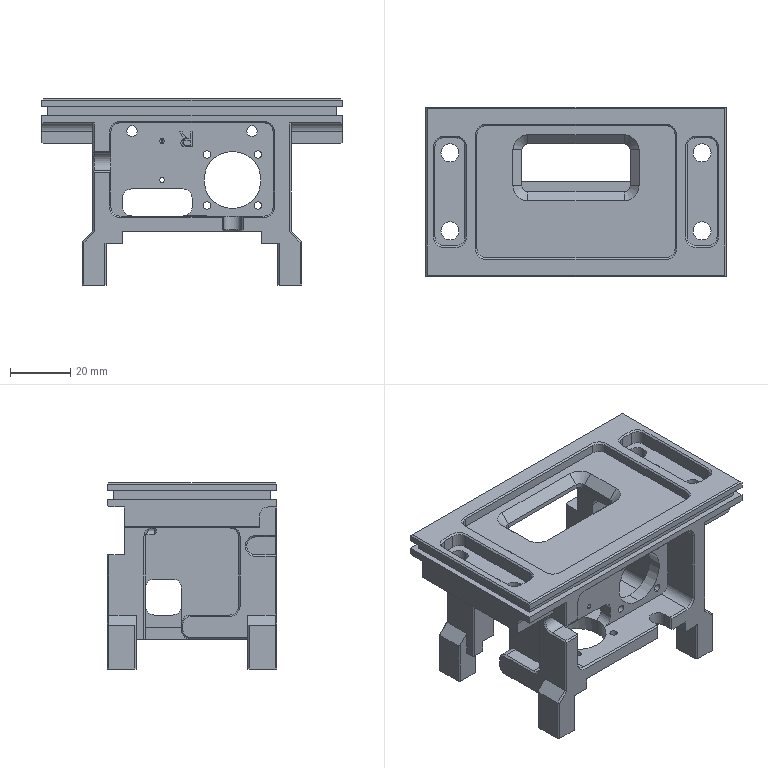NC program | Mastercam | posted with a generic post | part box 100 x 56.5 x 62 mm
Lines 34 to 1353 of 45570:
N260 T13 M6
N270 G0 G90 G17 G54 X-61.557 Y-50.411 A0. S5500 M3
N280 G43 H13 Z20. M8
N290 Z1.
N300 G1 Z-28.25 F600.
N310 X-62.09 Y-49.087 Z-28.374 F3000.
N320 G3 X-62.884 Y-47.884 Z-28.5 I-3.34 J-1.343
N330 G1 X-63.092 Y-47.603
N340 X-63.557 Y-46.951
N350 X-63.842 Y-46.52
N360 X-64.135 Y-46.037
N370 X-64.424 Y-45.51
N380 X-64.698 Y-44.943
N390 X-64.951 Y-44.341
N400 X-65.173 Y-43.718
N410 X-65.349 Y-43.127
N420 X-65.486 Y-42.577
N430 X-65.592 Y-42.064
N440 X-65.674 Y-41.586
N450 X-65.738 Y-41.138
N460 X-65.826 Y-40.34
N470 X-65.882 Y-39.609
N480 X-65.918 Y-38.931
N490 X-65.941 Y-38.291
N500 X-65.956 Y-37.678
N510 X-65.965 Y-37.084
N520 X-65.971 Y-36.505
N530 X-65.974 Y-35.935
N540 X-65.975 Y-35.371
N550 X-65.976 Y-34.813
N560 X-65.975 Y-34.258
N570 X-65.974 Y-33.705
N580 X-65.973 Y-33.153
N590 X-65.972 Y-32.603
N600 X-65.971 Y-32.052
N610 X-65.969 Y-31.502
N620 X-65.967 Y-30.953
N630 X-65.966 Y-30.403
N640 X-65.964 Y-29.853
N650 X-65.963 Y-29.304
N660 X-65.961 Y-28.754
N670 X-65.959 Y-28.205
N680 X-65.958 Y-27.655
N690 X-65.956 Y-27.105
N700 X-65.955 Y-26.556
N710 X-65.953 Y-26.006
N720 X-65.951 Y-25.456
N730 X-65.95 Y-24.906
N740 X-65.948 Y-24.357
N750 X-65.946 Y-23.807
N760 X-65.945 Y-23.257
N770 X-65.943 Y-22.707
N780 X-65.942 Y-22.157
N790 X-65.94 Y-21.607
N800 X-65.938 Y-21.057
N810 X-65.937 Y-20.507
N820 X-65.935 Y-19.957
N830 X-65.933 Y-19.407
N840 X-65.932 Y-18.857
N850 X-65.93 Y-18.307
N860 X-65.929 Y-17.757
N870 X-65.927 Y-17.207
N880 X-65.925 Y-16.656
N890 X-65.924 Y-16.106
N900 X-65.922 Y-15.556
N910 X-65.92 Y-15.006
N920 X-65.919 Y-14.456
N930 X-65.917 Y-13.905
N940 X-65.916 Y-13.355
N950 X-65.914 Y-12.805
N960 X-65.912 Y-12.254
N970 X-65.911 Y-11.704
N980 X-65.909 Y-11.153
N990 X-65.907 Y-10.603
N1000 X-65.906 Y-10.052
N1010 X-65.904 Y-9.502
N1020 X-65.903 Y-8.951
N1030 X-65.901 Y-8.401
N1040 X-65.899 Y-7.85
N1050 X-65.898 Y-7.3
N1060 X-65.896 Y-6.749
N1070 X-65.894 Y-6.199
N1080 X-65.893 Y-5.648
N1090 X-65.891 Y-5.097
N1100 X-65.89 Y-4.547
N1110 X-65.888 Y-3.996
N1120 X-65.886 Y-3.445
N1130 X-65.885 Y-2.895
N1140 X-65.883 Y-2.344
N1150 X-65.881 Y-1.793
N1160 X-65.88 Y-1.242
N1170 X-65.878 Y-.691
N1180 X-65.877 Y-.141
N1190 X-65.875 Y.41
N1200 X-65.873 Y.961
N1210 X-65.872 Y1.512
N1220 X-65.87 Y2.063
N1230 X-65.868 Y2.614
N1240 X-65.867 Y3.165
N1250 X-65.865 Y3.716
N1260 X-65.863 Y4.267
N1270 X-65.862 Y4.818
N1280 X-65.86 Y5.369
N1290 X-65.859 Y5.92
N1300 X-65.857 Y6.471
N1310 X-65.855 Y7.022
N1320 X-65.854 Y7.573
N1330 X-65.852 Y8.124
N1340 X-65.85 Y8.675
N1350 X-65.849 Y9.226
N1360 X-65.847 Y9.778
N1370 X-65.846 Y10.329
N1380 X-65.844 Y10.88
N1390 X-65.842 Y11.431
N1400 X-65.841 Y11.982
N1410 X-65.839 Y12.534
N1420 X-65.837 Y13.085
N1430 X-65.836 Y13.636
N1440 X-65.834 Y14.187
N1450 X-65.833 Y14.739
N1460 X-65.831 Y15.29
N1470 X-65.829 Y15.841
N1480 X-65.828 Y16.393
N1490 X-65.826 Y16.944
N1500 X-65.824 Y17.495
N1510 X-65.823 Y18.047
N1520 X-65.821 Y18.598
N1530 X-65.819 Y19.149
N1540 X-65.818 Y19.701
N1550 X-65.816 Y20.252
N1560 X-65.815 Y20.804
N1570 X-65.813 Y21.355
N1580 X-65.811 Y21.907
N1590 X-65.81 Y22.458
N1600 X-65.808 Y23.01
N1610 X-65.806 Y23.561
N1620 X-65.805 Y24.113
N1630 X-65.803 Y24.664
N1640 X-65.802 Y25.216
N1650 X-65.8 Y25.767
N1660 X-65.798 Y26.319
N1670 X-65.797 Y26.871
N1680 X-65.795 Y27.422
N1690 X-65.793 Y27.974
N1700 X-65.792 Y28.525
N1710 X-65.79 Y29.077
N1720 X-65.788 Y29.629
N1730 X-65.787 Y30.18
N1740 X-65.785 Y30.732
N1750 X-65.784 Y31.284
N1760 X-65.782 Y31.836
N1770 X-65.78 Y32.387
N1780 X-65.779 Y32.939
N1790 X-65.777 Y33.491
N1800 X-65.775 Y34.043
N1810 X-65.774 Y34.594
N1820 X-65.772 Y35.146
N1830 X-65.771 Y35.698
N1840 X-65.769 Y36.25
N1850 X-65.767 Y36.802
N1860 X-65.766 Y37.353
N1870 X-65.763 Y37.956
N1880 X-65.741 Y38.755
N1890 X-65.712 Y39.225
N1900 X-65.664 Y39.727
N1910 X-65.595 Y40.255
N1920 X-65.501 Y40.803
N1930 X-65.378 Y41.367
N1940 X-65.225 Y41.941
N1950 X-65.038 Y42.521
N1960 X-64.816 Y43.103
N1970 X-64.558 Y43.682
N1980 X-64.263 Y44.254
N1990 X-63.93 Y44.815
N2000 X-63.561 Y45.361
N2010 X-63.155 Y45.888
N2020 X-62.713 Y46.394
N2030 X-62.236 Y46.873
N2040 X-61.727 Y47.322
N2050 X-61.206 Y47.726
N2060 X-60.682 Y48.086
N2070 X-60.159 Y48.403
N2080 X-59.642 Y48.683
N2090 X-59.134 Y48.928
N2100 X-58.637 Y49.142
N2110 X-58.152 Y49.33
N2120 X-57.68 Y49.493
N2130 X-57.221 Y49.635
N2140 X-56.775 Y49.759
N2150 X-56.343 Y49.867
N2160 X-55.531 Y50.041
N2170 X-54.76 Y50.176
N2180 X-54.023 Y50.28
N2190 X-53.317 Y50.361
N2200 X-52.638 Y50.424
N2210 X-51.981 Y50.473
N2220 X-51.343 Y50.511
N2230 X-50.721 Y50.542
N2240 X-50.111 Y50.565
N2250 X-49.512 Y50.584
N2260 X-48.922 Y50.598
N2270 X-48.338 Y50.609
N2280 X-47.761 Y50.618
N2290 X-47.189 Y50.624
N2300 X-46.62 Y50.629
N2310 X-46.054 Y50.633
N2320 X-45.49 Y50.636
N2330 X-44.927 Y50.639
N2340 X-44.365 Y50.641
N2350 X-43.804 Y50.642
N2360 X-43.243 Y50.644
N2370 X-42.684 Y50.645
N2380 X-42.124 Y50.646
N2390 X-41.566 Y50.647
N2400 X-41.007
N2410 X-40.449 Y50.648
N2420 X-39.891
N2430 X-39.333
N2440 X-38.776 Y50.649
N2450 X-38.218
N2460 X-37.661
N2470 X-37.104
N2480 X-36.546
N2490 X-35.989 Y50.65
N2500 X-35.432
N2510 X-34.875
N2520 X-34.318
N2530 X-33.761
N2540 X-33.204
N2550 X-32.647
N2560 X-32.09
N2570 X-31.533
N2580 X-30.976
N2590 X-30.419
N2600 X-29.862
N2610 X-29.305
N2620 X-28.748
N2630 X-28.191
N2640 X-27.634
N2650 X-27.077
N2660 X-26.521
N2670 X-25.964
N2680 X-25.407
N2690 X-24.85
N2700 X-24.293
N2710 X-23.736
N2720 X-23.179
N2730 X-22.622
N2740 X-22.065
N2750 X-21.508
N2760 X-20.951
N2770 X-20.394
N2780 X-19.838
N2790 X-19.281
N2800 X-18.724
N2810 X-18.167
N2820 X-17.61
N2830 X-17.053
N2840 X-16.496
N2850 X-15.939
N2860 X-15.382
N2870 X-14.825
N2880 X-14.268
N2890 X-13.712
N2900 X-13.155
N2910 X-12.598
N2920 X-12.041
N2930 X-11.484
N2940 X-10.927
N2950 X-10.37
N2960 X-9.813
N2970 X-9.256
N2980 X-8.699
N2990 X-8.142
N3000 X-7.586
N3010 X-7.029
N3020 X-6.472
N3030 X-5.915
N3040 X-5.358
N3050 X-4.801
N3060 X-4.244
N3070 X-3.687
N3080 X-3.13
N3090 X-2.573
N3100 X-2.016
N3110 X-1.46
N3120 X-.903
N3130 X-.346
N3140 X.211
N3150 X.768
N3160 X1.325
N3170 X1.882
N3180 X2.439
N3190 X2.996
N3200 X3.553
N3210 X4.11
N3220 X4.667
N3230 X5.223
N3240 X5.78
N3250 X6.337
N3260 X6.894
N3270 X7.451
N3280 X8.008
N3290 X8.565
N3300 X9.122
N3310 X9.679
N3320 X10.236
N3330 X10.793
N3340 X11.349
N3350 X11.906
N3360 X12.463
N3370 X13.02
N3380 X13.577
N3390 X14.134
N3400 X14.691
N3410 X15.248
N3420 X15.805
N3430 X16.362
N3440 X16.919
N3450 X17.475
N3460 X18.032
N3470 X18.589
N3480 X19.146
N3490 X19.703
N3500 X20.26
N3510 X20.817
N3520 X21.374
N3530 X21.931
N3540 X22.488
N3550 X23.045
N3560 X23.601
N3570 X24.158
N3580 X24.715
N3590 X25.272
N3600 X25.829
N3610 X26.386
N3620 X26.943
N3630 X27.5
N3640 X28.057
N3650 X28.614
N3660 X29.171
N3670 X29.727
N3680 X30.284
N3690 X30.841
N3700 X31.398
N3710 X31.955
N3720 X32.512
N3730 X33.069
N3740 X33.626
N3750 X34.183
N3760 X34.74
N3770 X35.297
N3780 X35.853
N3790 X36.41
N3800 X36.967
N3810 X37.524
N3820 X38.081
N3830 X38.638
N3840 X39.195
N3850 X39.752
N3860 X40.309
N3870 X40.866
N3880 X41.423
N3890 X41.979
N3900 X42.536
N3910 X43.093
N3920 X43.65
N3930 X44.207
N3940 X44.764
N3950 X45.321
N3960 X45.878
N3970 X46.435
N3980 X46.992
N3990 X47.549
N4000 X48.106
N4010 X48.662
N4020 X49.219
N4030 X49.776
N4040 X50.333
N4050 X50.89
N4060 X51.447
N4070 X52.004
N4080 X52.602 Y50.649
N4090 X53.378 Y50.633
N4100 X53.831 Y50.61
N4110 X54.315 Y50.571
N4120 X54.825 Y50.513
N4130 X55.356 Y50.432
N4140 X55.903 Y50.326
N4150 X56.462 Y50.192
N4160 X57.028 Y50.026
N4170 X57.599 Y49.829
N4180 X58.169 Y49.597
N4190 X58.735 Y49.331
N4200 X59.292 Y49.028
N4210 X59.838 Y48.69
N4220 X60.369 Y48.315
N4230 X60.881 Y47.905
N4240 X61.37 Y47.46
N4250 X61.832 Y46.983
N4260 X62.253 Y46.49
N4270 X62.634 Y45.988
N4280 X62.975 Y45.483
N4290 X63.28 Y44.978
N4300 X63.552 Y44.478
N4310 X63.793 Y43.983
N4320 X64.006 Y43.498
N4330 X64.194 Y43.021
N4340 X64.36 Y42.556
N4350 X64.507 Y42.102
N4360 X64.636 Y41.659
N4370 X64.75 Y41.227
N4380 X64.936 Y40.413
N4390 X65.081 Y39.635
N4400 X65.196 Y38.891
N4410 X65.286 Y38.176
N4420 X65.358 Y37.487
N4430 X65.415 Y36.82
N4440 X65.46 Y36.172
N4450 X65.496 Y35.539
N4460 X65.526 Y34.92
N4470 X65.549 Y34.311
N4480 X65.568 Y33.712
N4490 X65.583 Y33.12
N4500 X65.596 Y32.534
N4510 X65.606 Y31.954
N4520 X65.614 Y31.378
N4530 X65.621 Y30.805
N4540 X65.626 Y30.235
N4550 X65.63 Y29.668
N4560 X65.634 Y29.102
N4570 X65.637 Y28.538
N4580 X65.639 Y27.975
N4590 X65.641 Y27.413
N4600 X65.643 Y26.853
N4610 X65.644 Y26.292
N4620 X65.645 Y25.733
N4630 X65.646 Y25.174
N4640 X65.647 Y24.615
N4650 Y24.057
N4660 X65.648 Y23.499
N4670 Y22.941
N4680 X65.649 Y22.383
N4690 Y21.826
N4700 Y21.268
N4710 Y20.711
N4720 Y20.154
N4730 Y19.596
N4740 X65.65 Y19.039
N4750 Y18.482
N4760 Y17.925
N4770 Y17.368
N4780 Y16.811
N4790 Y16.254
N4800 Y15.697
N4810 Y15.14
N4820 Y14.583
N4830 Y14.026
N4840 Y13.469
N4850 Y12.912
N4860 Y12.355
N4870 Y11.798
N4880 Y11.241
N4890 Y10.684
N4900 Y10.128
N4910 Y9.571
N4920 Y9.014
N4930 Y8.457
N4940 Y7.9
N4950 Y7.343
N4960 Y6.786
N4970 Y6.229
N4980 Y5.672
N4990 Y5.115
N5000 Y4.558
N5010 Y4.001
N5020 Y3.445
N5030 Y2.888
N5040 Y2.331
N5050 Y1.774
N5060 Y1.217
N5070 Y.66
N5080 Y.103
N5090 Y-.454
N5100 Y-1.011
N5110 Y-1.568
N5120 Y-2.125
N5130 Y-2.681
N5140 Y-3.238
N5150 Y-3.795
N5160 Y-4.352
N5170 Y-4.909
N5180 Y-5.466
N5190 Y-6.023
N5200 Y-6.58
N5210 Y-7.137
N5220 Y-7.694
N5230 Y-8.251
N5240 Y-8.807
N5250 Y-9.364
N5260 Y-9.921
N5270 Y-10.478
N5280 Y-11.035
N5290 Y-11.592
N5300 Y-12.149
N5310 Y-12.706
N5320 Y-13.263
N5330 Y-13.82
N5340 Y-14.377
N5350 Y-14.933
N5360 Y-15.49
N5370 Y-16.047
N5380 Y-16.604
N5390 Y-17.161
N5400 Y-17.718
N5410 Y-18.275
N5420 Y-18.832
N5430 Y-19.389
N5440 Y-19.946
N5450 Y-20.503
N5460 Y-21.06
N5470 Y-21.616
N5480 Y-22.173
N5490 Y-22.73
N5500 Y-23.287
N5510 Y-23.844
N5520 Y-24.401
N5530 Y-24.958
N5540 Y-25.515
N5550 Y-26.072
N5560 Y-26.629
N5570 Y-27.186
N5580 Y-27.742
N5590 Y-28.299
N5600 Y-28.856
N5610 Y-29.413
N5620 Y-29.97
N5630 Y-30.527
N5640 Y-31.084
N5650 Y-31.641
N5660 Y-32.198
N5670 Y-32.755
N5680 Y-33.312
N5690 Y-33.868
N5700 Y-34.425
N5710 Y-34.982
N5720 Y-35.539
N5730 Y-36.096
N5740 Y-36.653
N5750 Y-37.21
N5760 X65.646 Y-37.871
N5770 X65.618 Y-38.703
N5780 X65.583 Y-39.179
N5790 X65.531 Y-39.682
N5800 X65.457 Y-40.207
N5810 X65.358 Y-40.75
N5820 X65.232 Y-41.306
N5830 X65.075 Y-41.871
N5840 X64.887 Y-42.441
N5850 X64.665 Y-43.011
N5860 X64.408 Y-43.579
N5870 X64.116 Y-44.139
N5880 X63.787 Y-44.689
N5890 X63.422 Y-45.224
N5900 X63.022 Y-45.741
N5910 X62.587 Y-46.237
N5920 X62.117 Y-46.708
N5930 X61.628 Y-47.141
N5940 X61.128 Y-47.533
N5950 X60.623 Y-47.885
N5960 X60.118 Y-48.199
N5970 X59.616 Y-48.48
N5980 X59.119 Y-48.729
N5990 X58.631 Y-48.95
N6000 X58.152 Y-49.145
N6010 X57.684 Y-49.317
N6020 X57.226 Y-49.468
N6030 X56.78 Y-49.602
N6040 X56.345 Y-49.72
N6050 X55.921 Y-49.824
N6060 X55.121 Y-49.994
N6070 X54.356 Y-50.127
N6080 X53.624 Y-50.232
N6090 X52.919 Y-50.315
N6100 X52.238 Y-50.381
N6110 X51.578 Y-50.433
N6120 X50.936 Y-50.475
N6130 X50.309 Y-50.508
N6140 X49.693 Y-50.535
N6150 X49.089 Y-50.556
N6160 X48.492 Y-50.574
N6170 X47.903 Y-50.588
N6180 X47.319 Y-50.6
N6190 X46.74 Y-50.609
N6200 X46.165 Y-50.616
N6210 X45.594 Y-50.623
N6220 X45.025 Y-50.628
N6230 X44.458 Y-50.632
N6240 X43.893 Y-50.635
N6250 X43.329 Y-50.638
N6260 X42.767 Y-50.64
N6270 X42.206 Y-50.642
N6280 X41.645 Y-50.643
N6290 X41.085 Y-50.645
N6300 X40.526 Y-50.646
N6310 X39.967
N6320 X39.409 Y-50.647
N6330 X38.85 Y-50.648
N6340 X38.292
N6350 X37.735
N6360 X37.177 Y-50.649
N6370 X36.619
N6380 X36.062
N6390 X35.505
N6400 X34.947
N6410 X34.39
N6420 X33.833 Y-50.65
N6430 X33.276
N6440 X32.719
N6450 X32.162
N6460 X31.605
N6470 X31.048
N6480 X30.491
N6490 X29.934
N6500 X29.377
N6510 X28.82
N6520 X28.263
N6530 X27.706
N6540 X27.149
N6550 X26.592
N6560 X26.035
N6570 X25.478
N6580 X24.921
N6590 X24.364
N6600 X23.808
N6610 X23.251
N6620 X22.694
N6630 X22.137
N6640 X21.58
N6650 X21.023
N6660 X20.466
N6670 X19.909
N6680 X19.352
N6690 X18.795
N6700 X18.238
N6710 X17.682
N6720 X17.125
N6730 X16.568
N6740 X16.011
N6750 X15.454
N6760 X14.897
N6770 X14.34
N6780 X13.783
N6790 X13.226
N6800 X12.669
N6810 X12.112
N6820 X11.555
N6830 X10.999
N6840 X10.442
N6850 X9.885
N6860 X9.328
N6870 X8.771
N6880 X8.214
N6890 X7.657
N6900 X7.1
N6910 X6.543
N6920 X5.986
N6930 X5.429
N6940 X4.873
N6950 X4.316
N6960 X3.759
N6970 X3.202
N6980 X2.645
N6990 X2.088
N7000 X1.531
N7010 X.974
N7020 X.417
N7030 X-.14
N7040 X-.697
N7050 X-1.253
N7060 X-1.81
N7070 X-2.367
N7080 X-2.924
N7090 X-3.481
N7100 X-4.038
N7110 X-4.595
N7120 X-5.152
N7130 X-5.709
N7140 X-6.266
N7150 X-6.823
N7160 X-7.379
N7170 X-7.936
N7180 X-8.493
N7190 X-9.05
N7200 X-9.607
N7210 X-10.164
N7220 X-10.721
N7230 X-11.278
N7240 X-11.835
N7250 X-12.392
N7260 X-12.949
N7270 X-13.505
N7280 X-14.062
N7290 X-14.619
N7300 X-15.176
N7310 X-15.733
N7320 X-16.29
N7330 X-16.847
N7340 X-17.404
N7350 X-17.961
N7360 X-18.518
N7370 X-19.075
N7380 X-19.631
N7390 X-20.188
N7400 X-20.745
N7410 X-21.302
N7420 X-21.859
N7430 X-22.416
N7440 X-22.973
N7450 X-23.53
N7460 X-24.087
N7470 X-24.644
N7480 X-25.201
N7490 X-25.758
N7500 X-26.314
N7510 X-26.871
N7520 X-27.428
N7530 X-27.985
N7540 X-28.542
N7550 X-29.099
N7560 X-29.656
N7570 X-30.213
N7580 X-30.77
N7590 X-31.327
N7600 X-31.884
N7610 X-32.44
N7620 X-32.997
N7630 X-33.554
N7640 X-34.111
N7650 X-34.668
N7660 X-35.225
N7670 X-35.782
N7680 X-36.339
N7690 X-36.896
N7700 X-37.453
N7710 X-38.01
N7720 X-38.566
N7730 X-39.123
N7740 X-39.68
N7750 X-40.237
N7760 X-40.794
N7770 X-41.351
N7780 X-41.908
N7790 X-42.465
N7800 X-43.022
N7810 X-43.579
N7820 X-44.136
N7830 X-44.692
N7840 X-45.249
N7850 X-45.806
N7860 X-46.363
N7870 X-46.92
N7880 X-47.477
N7890 X-48.034
N7900 X-48.591
N7910 X-49.148
N7920 X-49.705
N7930 X-50.262
N7940 X-50.818
N7950 X-51.375
N7960 X-51.932
N7970 X-52.515
N7980 X-53.27 Y-50.637
N7990 X-53.714 Y-50.617
N8000 X-54.191 Y-50.582
N8010 X-54.695 Y-50.529
N8020 X-55.221 Y-50.455
N8030 X-55.809 Y-50.345
N8040 X-56.451 Y-50.186
N8050 X-57.077 Y-49.989
N8060 X-57.687 Y-49.755
N8070 X-58.281 Y-49.484
N8080 X-58.857 Y-49.178
N8090 X-59.414 Y-48.837
N8100 X-59.948 Y-48.462
N8110 X-60.455 Y-48.059
N8120 X-60.931 Y-47.632
N8130 X-61.376 Y-47.184
N8140 X-61.787 Y-46.722
N8150 X-62.164 Y-46.251
N8160 X-62.509 Y-45.771
N8170 X-62.823 Y-45.289
N8180 X-63.108 Y-44.805
N8190 X-63.364 Y-44.323
N8200 X-63.595 Y-43.845
N8210 X-63.801 Y-43.374
N8220 X-63.986 Y-42.909
N8230 X-64.15 Y-42.452
N8240 X-64.297 Y-42.005
N8250 X-64.427 Y-41.566
N8260 X-64.543 Y-41.137
N8270 X-64.733 Y-40.325
N8280 X-64.884 Y-39.546
N8290 X-65.003 Y-38.798
N8300 X-65.098 Y-38.078
N8310 X-65.172 Y-37.383
N8320 X-65.231 Y-36.711
N8330 X-65.278 Y-36.057
N8340 X-65.315 Y-35.42
N8350 X-65.345 Y-34.796
N8360 X-65.368 Y-34.184
N8370 X-65.387 Y-33.582
N8380 X-65.402 Y-32.988
N8390 X-65.413 Y-32.4
N8400 X-65.422 Y-31.818
N8410 X-65.43 Y-31.24
N8420 X-65.435 Y-30.666
N8430 X-65.439 Y-30.095
N8440 X-65.442 Y-29.527
N8450 X-65.444 Y-28.961
N8460 X-65.446 Y-28.396
N8470 X-65.447 Y-27.833
N8480 Y-27.271
N8490 Y-26.71
N8500 Y-26.149
N8510 Y-25.589
N8520 X-65.446 Y-25.03
N8530 X-65.445 Y-24.471
N8540 X-65.444 Y-23.913
N8550 X-65.443 Y-23.355
N8560 X-65.442 Y-22.797
N8570 X-65.44 Y-22.239
N8580 X-65.439 Y-21.682
N8590 X-65.438 Y-21.124
N8600 X-65.436 Y-20.567
N8610 X-65.435 Y-20.009
N8620 X-65.433 Y-19.452
N8630 X-65.431 Y-18.895
N8640 X-65.43 Y-18.338
N8650 X-65.428 Y-17.781
N8660 X-65.427 Y-17.224
N8670 X-65.425 Y-16.667
N8680 X-65.424 Y-16.11
N8690 X-65.422 Y-15.553
N8700 X-65.42 Y-14.996
N8710 X-65.419 Y-14.439
N8720 X-65.417 Y-13.882
N8730 X-65.415 Y-13.325
N8740 X-65.414 Y-12.768
N8750 X-65.412 Y-12.211
N8760 X-65.41 Y-11.654
N8770 X-65.409 Y-11.097
N8780 X-65.407 Y-10.54
N8790 X-65.406 Y-9.983
N8800 X-65.404 Y-9.426
N8810 X-65.402 Y-8.869
N8820 X-65.401 Y-8.312
N8830 X-65.399 Y-7.756
N8840 X-65.397 Y-7.199
N8850 X-65.396 Y-6.642
N8860 X-65.394 Y-6.085
N8870 X-65.392 Y-5.528
N8880 X-65.391 Y-4.971
N8890 X-65.389 Y-4.414
N8900 X-65.387 Y-3.857
N8910 X-65.386 Y-3.3
N8920 X-65.384 Y-2.743
N8930 X-65.383 Y-2.186
N8940 X-65.381 Y-1.63
N8950 X-65.379 Y-1.073
N8960 X-65.378 Y-.516
N8970 X-65.376 Y.041
N8980 X-65.374 Y.598
N8990 X-65.373 Y1.155
N9000 X-65.371 Y1.712
N9010 X-65.369 Y2.269
N9020 X-65.368 Y2.826
N9030 X-65.366 Y3.383
N9040 X-65.364 Y3.94
N9050 X-65.363 Y4.496
N9060 X-65.361 Y5.053
N9070 X-65.359 Y5.61
N9080 X-65.358 Y6.167
N9090 X-65.356 Y6.724
N9100 X-65.355 Y7.281
N9110 X-65.353 Y7.838
N9120 X-65.351 Y8.395
N9130 X-65.35 Y8.952
N9140 X-65.348 Y9.509
N9150 X-65.346 Y10.066
N9160 X-65.345 Y10.622
N9170 X-65.343 Y11.179
N9180 X-65.341 Y11.736
N9190 X-65.34 Y12.293
N9200 X-65.338 Y12.85
N9210 X-65.336 Y13.407
N9220 X-65.335 Y13.964
N9230 X-65.333 Y14.521
N9240 X-65.331 Y15.078
N9250 X-65.33 Y15.635
N9260 X-65.328 Y16.192
N9270 X-65.327 Y16.748
N9280 X-65.325 Y17.305
N9290 X-65.323 Y17.862
N9300 X-65.322 Y18.419
N9310 X-65.32 Y18.976
N9320 X-65.318 Y19.533
N9330 X-65.317 Y20.09
N9340 X-65.315 Y20.647
N9350 X-65.313 Y21.204
N9360 X-65.312 Y21.761
N9370 X-65.31 Y22.318
N9380 X-65.308 Y22.874
N9390 X-65.307 Y23.431
N9400 X-65.305 Y23.988
N9410 X-65.304 Y24.545
N9420 X-65.302 Y25.102
N9430 X-65.3 Y25.659
N9440 X-65.299 Y26.216
N9450 X-65.297 Y26.773
N9460 X-65.295 Y27.33
N9470 X-65.294 Y27.887
N9480 X-65.292 Y28.443
N9490 X-65.29 Y29.
N9500 X-65.289 Y29.557
N9510 X-65.287 Y30.114
N9520 X-65.285 Y30.671
N9530 X-65.284 Y31.228
N9540 X-65.282 Y31.785
N9550 X-65.28 Y32.342
N9560 X-65.279 Y32.899
N9570 X-65.277 Y33.456
N9580 X-65.276 Y34.013
N9590 X-65.274 Y34.57
N9600 X-65.272 Y35.132
N9610 X-65.269 Y35.722
N9620 X-65.259 Y36.383
N9630 X-65.231 Y37.133
N9640 X-65.204 Y37.555
N9650 X-65.165 Y38.001
N9660 X-65.111 Y38.477
N9670 X-65.038 Y38.977
N9680 X-64.941 Y39.503
N9690 X-64.817 Y40.047
N9700 X-64.661 Y40.613
N9710 X-64.472 Y41.188
N9720 X-64.247 Y41.765
N9730 X-63.989 Y42.333
N9740 X-63.699 Y42.888
N9750 X-63.379 Y43.425
N9760 X-63.032 Y43.94
N9770 X-62.662 Y44.431
N9780 X-62.271 Y44.896
N9790 X-61.862 Y45.334
N9800 X-61.435 Y45.748
N9810 X-61.003 Y46.129
N9820 X-60.558 Y46.486
N9830 X-60.112 Y46.813
N9840 X-59.658 Y47.118
N9850 X-59.206 Y47.396
N9860 X-58.75 Y47.653
N9870 X-58.3 Y47.886
N9880 X-57.85 Y48.1
N9890 X-57.407 Y48.294
N9900 X-56.966 Y48.471
N9910 X-56.534 Y48.631
N9920 X-56.106 Y48.777
N9930 X-55.687 Y48.908
N9940 X-54.883 Y49.131
N9950 X-54.105 Y49.315
N9960 X-53.35 Y49.465
N9970 X-52.619 Y49.588
N9980 X-51.91 Y49.689
N9990 X-51.221 Y49.772
N100 X-50.55 Y49.839
N110 X-49.895 Y49.895
N120 X-49.255 Y49.94
N130 X-48.627 Y49.977
N140 X-48.011 Y50.007
N150 X-47.404 Y50.032
N160 X-46.805 Y50.052
N170 X-46.213 Y50.069
N180 X-45.627 Y50.083
N190 X-45.045 Y50.095
N200 X-44.468 Y50.104
N210 X-43.894 Y50.112
N220 X-43.323 Y50.118
N230 X-42.754 Y50.124
N240 X-42.187 Y50.128
N250 X-41.622 Y50.132
N260 X-41.058 Y50.135
N270 X-40.495 Y50.138
N280 X-39.933 Y50.14
N290 X-39.373 Y50.142
N300 X-38.812 Y50.143
N310 X-38.253 Y50.144
N320 X-37.693 Y50.145
N330 X-37.135 Y50.146
N340 X-36.576 Y50.147
N350 X-36.018
N360 X-35.46 Y50.148
N370 X-34.902
N380 X-34.345
N390 X-33.787 Y50.149
N400 X-33.23
N410 X-32.672
N420 X-32.115
N430 X-31.558
N440 X-31.001
N450 X-30.443 Y50.15
N460 X-29.886
N470 X-29.329
N480 X-28.772
N490 X-28.215
N500 X-27.658
N510 X-27.101
N520 X-26.544
N530 X-25.987
N540 X-25.43
N550 X-24.873
N560 X-24.316
N570 X-23.76
N580 X-23.203
N590 X-22.646
N600 X-22.089
N610 X-21.532
N620 X-20.975
N630 X-20.418
N640 X-19.861
N650 X-19.304
N660 X-18.747
N670 X-18.19
N680 X-17.633
N690 X-17.077
N700 X-16.52
N710 X-15.963
N720 X-15.406
N730 X-14.849
N740 X-14.292
N750 X-13.735
N760 X-13.178
N770 X-12.621
N780 X-12.064
N790 X-11.507
N800 X-10.95
N810 X-10.394
N820 X-9.837
N830 X-9.28
N840 X-8.723
N850 X-8.166
N860 X-7.609
N870 X-7.052
N880 X-6.495
N890 X-5.938
N900 X-5.381
N910 X-4.824
N920 X-4.268
N930 X-3.711
N940 X-3.154
N950 X-2.597
N960 X-2.04
N970 X-1.483
N980 X-.926
N990 X-.369
N1000 X.188
N1010 X.745
N1020 X1.302
N1030 X1.858
N1040 X2.415
N1050 X2.972
N1060 X3.529
N1070 X4.086
N1080 X4.643
N1090 X5.2
N1100 X5.757
N1110 X6.314
N1120 X6.871
N1130 X7.428
N1140 X7.984
N1150 X8.541
N1160 X9.098
N1170 X9.655
N1180 X10.212
N1190 X10.769
N1200 X11.326
N1210 X11.883
N1220 X12.44
N1230 X12.997
N1240 X13.554
N1250 X14.11
N1260 X14.667
N1270 X15.224
N1280 X15.781
N1290 X16.338
N1300 X16.895
N1310 X17.452
N1320 X18.009
N1330 X18.566
N1340 X19.123
N1350 X19.68
N1360 X20.237
N1370 X20.793
N1380 X21.35
N1390 X21.907
N1400 X22.464
N1410 X23.021
N1420 X23.578
N1430 X24.135
N1440 X24.692
N1450 X25.249
N1460 X25.806
N1470 X26.363
N1480 X26.919
N1490 X27.476
N1500 X28.033
N1510 X28.59
N1520 X29.147
N1530 X29.704
N1540 X30.261
N1550 X30.818
N1560 X31.375
N1570 X31.932
N1580 X32.489
N1590 X33.045
N1600 X33.602
N1610 X34.159
N1620 X34.716
N1630 X35.273
N1640 X35.83
N1650 X36.387
N1660 X36.944
N1670 X37.501
N1680 X38.058
N1690 X38.615
N1700 X39.171
N1710 X39.728
N1720 X40.285
N1730 X40.842
N1740 X41.399
N1750 X41.956
N1760 X42.513
N1770 X43.07
N1780 X43.627
N1790 X44.184
N1800 X44.741
N1810 X45.297
N1820 X45.854
N1830 X46.411
N1840 X46.968
N1850 X47.525
N1860 X48.082
N1870 X48.639
N1880 X49.196
N1890 X49.755
N1900 X50.338 Y50.149
N1910 X50.981 Y50.142
N1920 X51.703 Y50.122
N1930 X52.519 Y50.073
N1940 X52.972 Y50.031
N1950 X53.454 Y49.971
N1960 X53.96 Y49.892
N1970 X54.492 Y49.788
N1980 X55.044 Y49.656
N1990 X55.613 Y49.49
N2000 X56.188 Y49.291
N2010 X56.76 Y49.059
N2020 X57.32 Y48.795
N2030 X57.865 Y48.501
N2040 X58.393 Y48.178
N2050 X58.898 Y47.831
N2060 X59.379 Y47.461
N2070 X59.835 Y47.072
N2080 X60.264 Y46.667
N2090 X60.671 Y46.245
N2100 X61.046 Y45.817
N2110 X61.397 Y45.379
N2120 X61.72 Y44.938
N2130 X62.022 Y44.491
N2140 X62.298 Y44.045
N2150 X62.554 Y43.595
N2160 X62.786 Y43.151
N2170 X63.001 Y42.705
N2180 X63.196 Y42.268
N2190 X63.375 Y41.831
N2200 X63.537 Y41.403
N2210 X63.685 Y40.978
N2220 X63.819 Y40.562
N2230 X64.048 Y39.763
N2240 X64.237 Y38.987
N2250 X64.394 Y38.234
N2260 X64.524 Y37.504
N2270 X64.631 Y36.795
N2280 X64.719 Y36.105
N2290 X64.792 Y35.433
N2300 X64.853 Y34.777
N2310 X64.903 Y34.134
N2320 X64.944 Y33.503
N2330 X64.979 Y32.884
N2340 X65.007 Y32.273
N2350 X65.031 Y31.671
N2360 X65.051 Y31.075
N2370 X65.067 Y30.485
N2380 X65.081 Y29.901
N2390 X65.093 Y29.32
N2400 X65.102 Y28.744
N2410 X65.11 Y28.17
N2420 X65.117 Y27.599
N2430 X65.122 Y27.03
N2440 X65.127 Y26.463
N2450 X65.131 Y25.898
N2460 X65.134 Y25.334
N2470 X65.137 Y24.772
N2480 X65.139 Y24.21
N2490 X65.141 Y23.649
N2500 X65.142 Y23.088
N2510 X65.144 Y22.529
N2520 X65.145 Y21.969
N2530 X65.146 Y21.41
N2540 Y20.852
N2550 X65.147 Y20.293
N2560 Y19.735
N2570 X65.148 Y19.178
N2580 Y18.62
N2590 X65.149 Y18.062
N2600 Y17.505
N2610 Y16.947
N2620 Y16.39
N2630 Y15.833
N2640 Y15.276
N2650 Y14.719
N2660 X65.15 Y14.161
N2670 Y13.604
N2680 Y13.047
N2690 Y12.49
N2700 Y11.933
N2710 Y11.376
N2720 Y10.819
N2730 Y10.262
N2740 Y9.705
N2750 Y9.148
N2760 Y8.591
N2770 Y8.034
N2780 Y7.478
N2790 Y6.921
N2800 Y6.364
N2810 Y5.807
N2820 Y5.25
N2830 Y4.693
N2840 Y4.136
N2850 Y3.579
N2860 Y3.022
N2870 Y2.465
N2880 Y1.908
N2890 Y1.351
N2900 Y.794
N2910 Y.238
N2920 Y-.319
N2930 Y-.876
N2940 Y-1.433
N2950 Y-1.99
N2960 Y-2.547
N2970 Y-3.104
N2980 Y-3.661
N2990 Y-4.218
N3000 Y-4.775
N3010 Y-5.332
N3020 Y-5.888
N3030 Y-6.445
N3040 Y-7.002
N3050 Y-7.559
N3060 Y-8.116
N3070 Y-8.673
N3080 Y-9.23
N3090 Y-9.787
N3100 Y-10.344
N3110 Y-10.901
N3120 Y-11.458
N3130 Y-12.014
N3140 Y-12.571
N3150 Y-13.128
N3160 Y-13.685
N3170 Y-14.242
N3180 Y-14.799
N3190 Y-15.356
N3200 Y-15.913
N3210 Y-16.47
N3220 Y-17.027
N3230 Y-17.584
N3240 Y-18.141
N3250 Y-18.697
N3260 Y-19.254
N3270 Y-19.811
N3280 Y-20.368
N3290 Y-20.925
N3300 Y-21.482
N3310 Y-22.039
N3320 Y-22.596
N3330 Y-23.153
N3340 Y-23.71
N3350 Y-24.267
N3360 Y-24.823
N3370 Y-25.38
N3380 Y-25.937
N3390 Y-26.494
N3400 Y-27.051
N3410 Y-27.608
N3420 Y-28.165
N3430 Y-28.722
N3440 Y-29.279
N3450 Y-29.836
N3460 Y-30.393
N3470 Y-30.949
N3480 Y-31.506
N3490 Y-32.063
N3500 Y-32.62
N3510 Y-33.177
N3520 Y-33.734
N3530 Y-34.291
N3540 Y-34.853
N3550 X65.148 Y-35.447